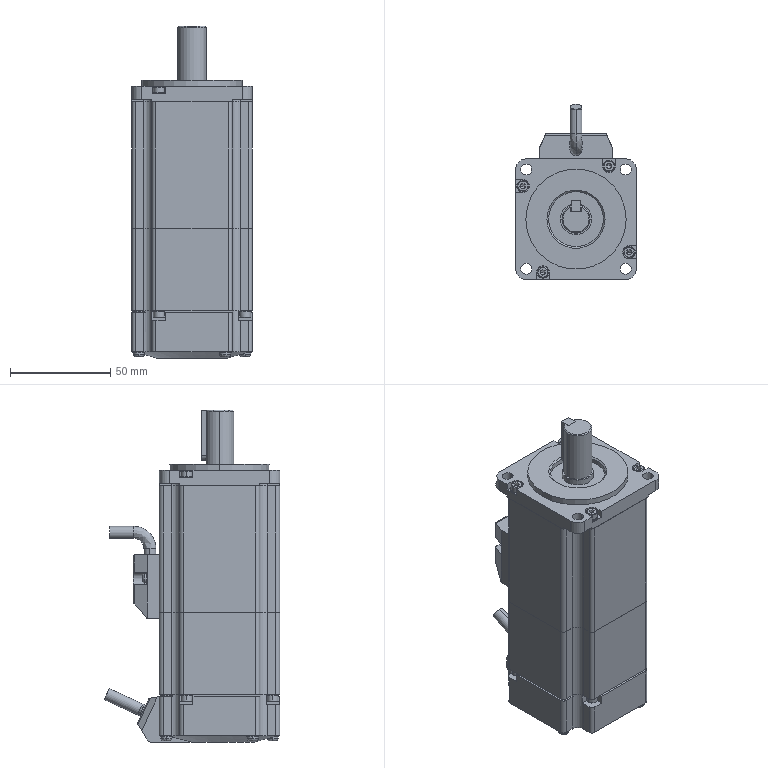Part | STEP file | C20604RS (Delta 400W) servo motor | 1 solid | 583 faces | box 60 x 87.491 x 165.5 mm | volume 457978 mm3 | plane 370 | cylinder 155 | cone 40 | spline 18 | commonest cylinder face diameters 5.5 x32 6 x32 4 x25 8 x16 2 x11 4.5 x8